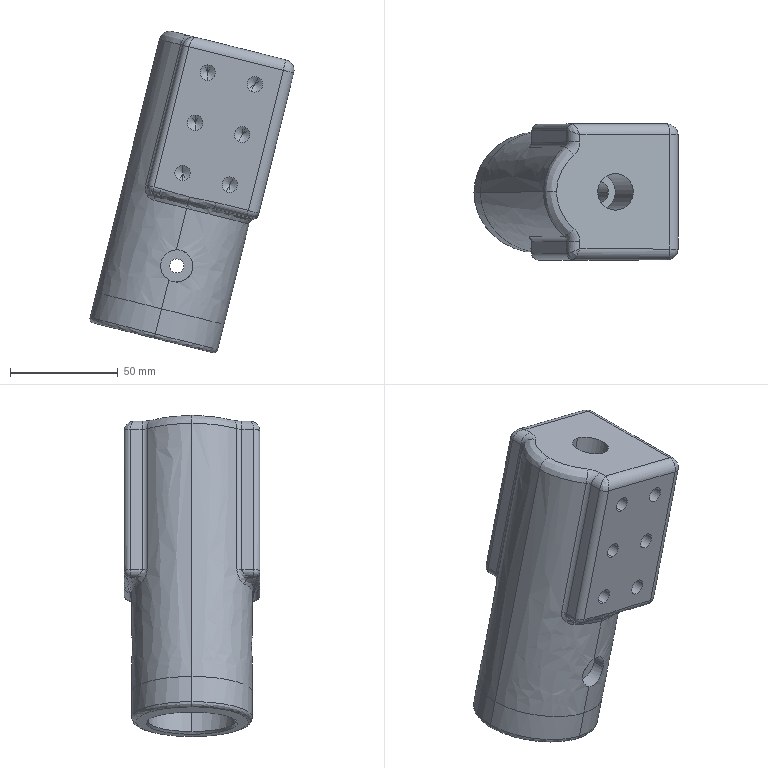Part | SolidWorks | features BaseBody 1 | 1 solid | 155 faces | box 94.672 x 63 x 149.112 mm | volume 379020 mm3 | cylinder 74 | spline 28 | cone 26 | plane 19 | torus 4 | sphere 4 | commonest cylinder face diameters 7.2 x24 6 x12 10 x11 6.5 x4 10.5 x4 14 x4